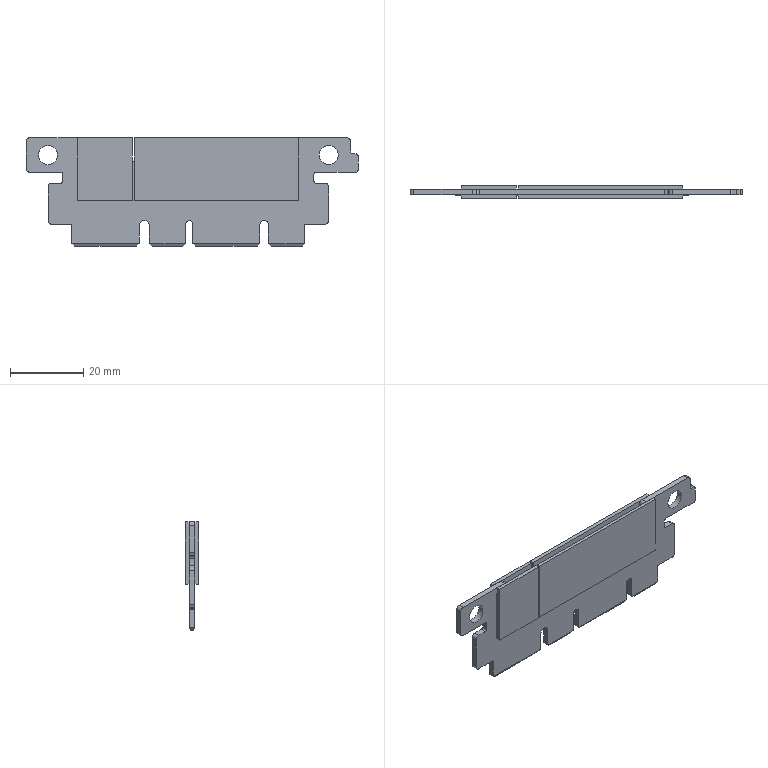Part | SolidWorks | features BaseBody 1, ICE 1, Split 1 | 5 solids | 100 faces | box 90.5 x 3.57 x 29.5 mm | volume 4915 mm3 | plane 73 | cylinder 27 | commonest cylinder face diameters 2 x11 1 x7 5.2 x4 0.6 x2 1.95 x1 2.25 x1